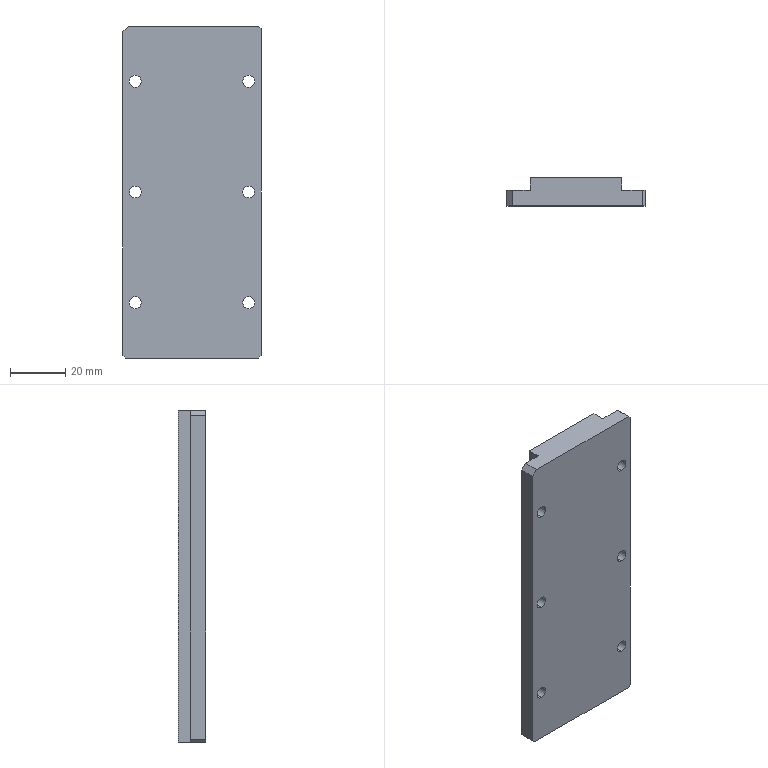Part | SolidWorks | features BaseBody 1 | 1 solid | 61 faces | box 50 x 10.1 x 120 mm | volume 50542 mm3 | plane 33 | cylinder 24 | spline 4 | commonest cylinder face diameters 4.3 x12 7.6 x12